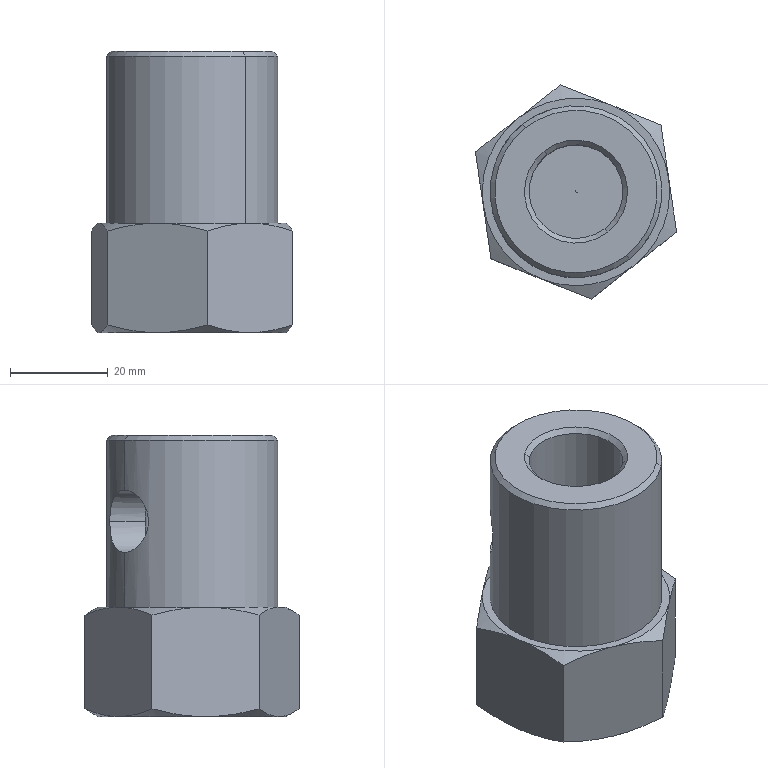Part | SolidWorks | features BaseBody 1 | 1 solid | 38 faces | box 41.191 x 43.879 x 57.6 mm | volume 49620 mm3 | cone 20 | plane 10 | cylinder 8 | commonest cylinder face diameters 10.56 x2 12.8 x2 19.2 x2 35.2 x2